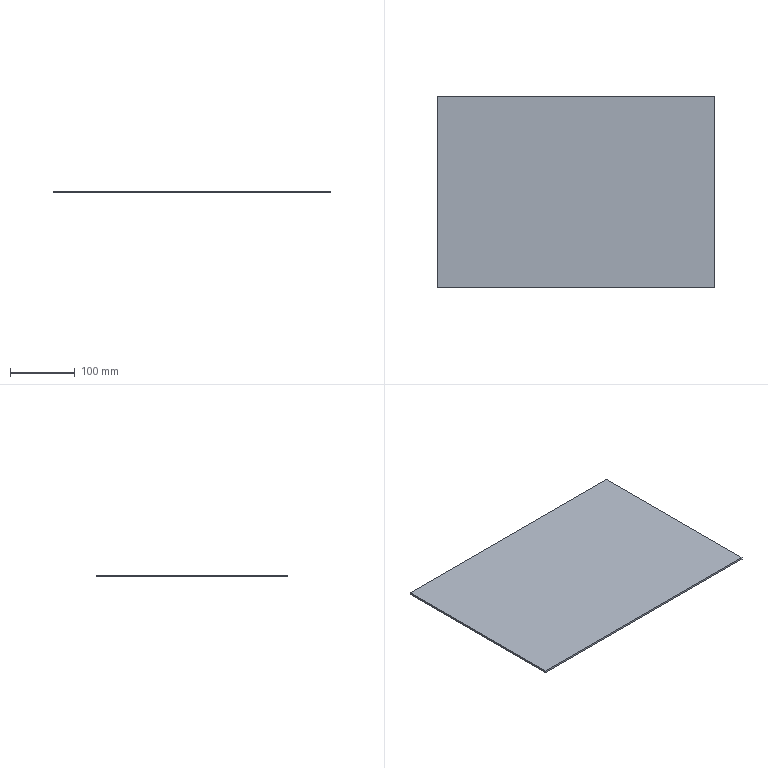Part | NX | features BREP 1 | 1 solid | 6 faces | box 429 x 296 x 3 mm | volume 380952 mm3 | plane 6
STEP:
#1=CARTESIAN_POINT('',(-214.5,148.,-1.5));
#2=VERTEX_POINT('',#1);
#3=CARTESIAN_POINT('',(-214.5,-148.,-1.5));
#4=VERTEX_POINT('',#3);
#5=CARTESIAN_POINT('',(-214.5,-148.,-1.5));
#6=DIRECTION('',(0.,-1.,0.));
#7=VECTOR('',#6,1000.);
#8=LINE('',#5,#7);
#9=EDGE_CURVE('',#2,#4,#8,.T.);
#10=ORIENTED_EDGE('',*,*,#9,.T.);
#11=CARTESIAN_POINT('',(-214.5,-148.,1.5));
#12=VERTEX_POINT('',#11);
#13=CARTESIAN_POINT('',(-214.5,-148.,1.5));
#14=DIRECTION('',(0.,0.,-1.));
#15=VECTOR('',#14,1000.);
#16=LINE('',#13,#15);
#17=EDGE_CURVE('',#12,#4,#16,.T.);
#18=ORIENTED_EDGE('',*,*,#17,.F.);
#19=CARTESIAN_POINT('',(-214.5,148.,1.5));
#20=VERTEX_POINT('',#19);
#21=CARTESIAN_POINT('',(-214.5,-148.,1.5));
#22=DIRECTION('',(0.,-1.,0.));
#23=VECTOR('',#22,1000.);
#24=LINE('',#21,#23);
#25=EDGE_CURVE('',#20,#12,#24,.T.);
#26=ORIENTED_EDGE('',*,*,#25,.F.);
#27=CARTESIAN_POINT('',(-214.5,148.,1.5));
#28=DIRECTION('',(0.,0.,-1.));
#29=VECTOR('',#28,1000.);
#30=LINE('',#27,#29);
#31=EDGE_CURVE('',#20,#2,#30,.T.);
#32=ORIENTED_EDGE('',*,*,#31,.T.);
#33=EDGE_LOOP('',(#10,#18,#26,#32));
#34=FACE_BOUND('',#33,.T.);
#35=CARTESIAN_POINT('',(-214.5,-148.,1.5));
#36=DIRECTION('',(-1.,0.,0.));
#37=DIRECTION('',(0.,0.,1.));
#38=AXIS2_PLACEMENT_3D('',#35,#36,#37);
#39=PLANE('',#38);
#40=ADVANCED_FACE('',(#34),#39,.T.);
#41=CARTESIAN_POINT('',(214.5,148.,-1.5));
#42=VERTEX_POINT('',#41);
#43=CARTESIAN_POINT('',(-214.5,148.,-1.5));
#44=DIRECTION('',(-1.,0.,0.));
#45=VECTOR('',#44,1000.);
#46=LINE('',#43,#45);
#47=EDGE_CURVE('',#42,#2,#46,.T.);
#48=ORIENTED_EDGE('',*,*,#47,.T.);
#49=ORIENTED_EDGE('',*,*,#31,.F.);
#50=CARTESIAN_POINT('',(214.5,148.,1.5));
#51=VERTEX_POINT('',#50);
#52=CARTESIAN_POINT('',(-214.5,148.,1.5));
#53=DIRECTION('',(-1.,0.,0.));
#54=VECTOR('',#53,1000.);
#55=LINE('',#52,#54);
#56=EDGE_CURVE('',#51,#20,#55,.T.);
#57=ORIENTED_EDGE('',*,*,#56,.F.);
#58=CARTESIAN_POINT('',(214.5,148.,1.5));
#59=DIRECTION('',(0.,0.,-1.));
#60=VECTOR('',#59,1000.);
#61=LINE('',#58,#60);
#62=EDGE_CURVE('',#51,#42,#61,.T.);
#63=ORIENTED_EDGE('',*,*,#62,.T.);
#64=EDGE_LOOP('',(#48,#49,#57,#63));
#65=FACE_BOUND('',#64,.T.);
#66=CARTESIAN_POINT('',(-214.5,148.,1.5));
#67=DIRECTION('',(0.,1.,0.));
#68=DIRECTION('',(1.,0.,0.));
#69=AXIS2_PLACEMENT_3D('',#66,#67,#68);
#70=PLANE('',#69);
#71=ADVANCED_FACE('',(#65),#70,.T.);
#72=CARTESIAN_POINT('',(214.5,-148.,-1.5));
#73=VERTEX_POINT('',#72);
#74=CARTESIAN_POINT('',(214.5,-148.,-1.5));
#75=DIRECTION('',(0.,1.,0.));
#76=VECTOR('',#75,1000.);
#77=LINE('',#74,#76);
#78=EDGE_CURVE('',#73,#42,#77,.T.);
#79=ORIENTED_EDGE('',*,*,#78,.T.);
#80=ORIENTED_EDGE('',*,*,#62,.F.);
#81=CARTESIAN_POINT('',(214.5,-148.,1.5));
#82=VERTEX_POINT('',#81);
#83=CARTESIAN_POINT('',(214.5,-148.,1.5));
#84=DIRECTION('',(0.,1.,0.));
#85=VECTOR('',#84,1000.);
#86=LINE('',#83,#85);
#87=EDGE_CURVE('',#82,#51,#86,.T.);
#88=ORIENTED_EDGE('',*,*,#87,.F.);
#89=CARTESIAN_POINT('',(214.5,-148.,1.5));
#90=DIRECTION('',(0.,0.,-1.));
#91=VECTOR('',#90,1000.);
#92=LINE('',#89,#91);
#93=EDGE_CURVE('',#82,#73,#92,.T.);
#94=ORIENTED_EDGE('',*,*,#93,.T.);
#95=EDGE_LOOP('',(#79,#80,#88,#94));
#96=FACE_BOUND('',#95,.T.);
#97=CARTESIAN_POINT('',(214.5,-148.,1.5));
#98=DIRECTION('',(1.,0.,0.));
#99=DIRECTION('',(0.,1.,0.));
#100=AXIS2_PLACEMENT_3D('',#97,#98,#99);
#101=PLANE('',#100);
#102=ADVANCED_FACE('',(#96),#101,.T.);
#103=CARTESIAN_POINT('',(-214.5,-148.,-1.5));
#104=DIRECTION('',(1.,0.,0.));
#105=VECTOR('',#104,1000.);
#106=LINE('',#103,#105);
#107=EDGE_CURVE('',#4,#73,#106,.T.);
#108=ORIENTED_EDGE('',*,*,#107,.T.);
#109=ORIENTED_EDGE('',*,*,#93,.F.);
#110=CARTESIAN_POINT('',(-214.5,-148.,1.5));
#111=DIRECTION('',(1.,0.,0.));
#112=VECTOR('',#111,1000.);
#113=LINE('',#110,#112);
#114=EDGE_CURVE('',#12,#82,#113,.T.);
#115=ORIENTED_EDGE('',*,*,#114,.F.);
#116=ORIENTED_EDGE('',*,*,#17,.T.);
#117=EDGE_LOOP('',(#108,#109,#115,#116));
#118=FACE_BOUND('',#117,.T.);
#119=CARTESIAN_POINT('',(-214.5,-148.,1.5));
#120=DIRECTION('',(0.,-1.,0.));
#121=DIRECTION('',(0.,0.,-1.));
#122=AXIS2_PLACEMENT_3D('',#119,#120,#121);
#123=PLANE('',#122);
#124=ADVANCED_FACE('',(#118),#123,.T.);
#125=ORIENTED_EDGE('',*,*,#25,.T.);
#126=ORIENTED_EDGE('',*,*,#114,.T.);
#127=ORIENTED_EDGE('',*,*,#87,.T.);
#128=ORIENTED_EDGE('',*,*,#56,.T.);
#129=EDGE_LOOP('',(#125,#126,#127,#128));
#130=FACE_BOUND('',#129,.T.);
#131=CARTESIAN_POINT('',(0.,0.,1.5));
#132=DIRECTION('',(0.,0.,1.));
#133=DIRECTION('',(1.,0.,0.));
#134=AXIS2_PLACEMENT_3D('',#131,#132,#133);
#135=PLANE('',#134);
#136=ADVANCED_FACE('',(#130),#135,.T.);
#137=ORIENTED_EDGE('',*,*,#9,.F.);
#138=ORIENTED_EDGE('',*,*,#47,.F.);
#139=ORIENTED_EDGE('',*,*,#78,.F.);
#140=ORIENTED_EDGE('',*,*,#107,.F.);
#141=EDGE_LOOP('',(#137,#138,#139,#140));
#142=FACE_BOUND('',#141,.T.);
#143=CARTESIAN_POINT('',(0.,0.,-1.5));
#144=DIRECTION('',(0.,0.,1.));
#145=DIRECTION('',(1.,0.,0.));
#146=AXIS2_PLACEMENT_3D('',#143,#144,#145);
#147=PLANE('',#146);
#148=ADVANCED_FACE('',(#142),#147,.F.);
#149=CLOSED_SHELL('',(#40,#71,#102,#124,#136,#148));
#150=MANIFOLD_SOLID_BREP('',#149);
#151=(LENGTH_UNIT()NAMED_UNIT(*)SI_UNIT(.MILLI.,.METRE.));
#152=UNCERTAINTY_MEASURE_WITH_UNIT(LENGTH_MEASURE(0.00001),#151,'','');
#153=(NAMED_UNIT(*)PLANE_ANGLE_UNIT()SI_UNIT($,.RADIAN.));
#154=(NAMED_UNIT(*)SI_UNIT($,.STERADIAN.)SOLID_ANGLE_UNIT());
#155=(GEOMETRIC_REPRESENTATION_CONTEXT(3)GLOBAL_UNCERTAINTY_ASSIGNED_CONTEXT((#152))GLOBAL_UNIT_ASSIGNED_CONTEXT((#151,#153,#154))REPRESENTATION_CONTEXT('',''));
#156=ADVANCED_BREP_SHAPE_REPRESENTATION('',(#150),#155);